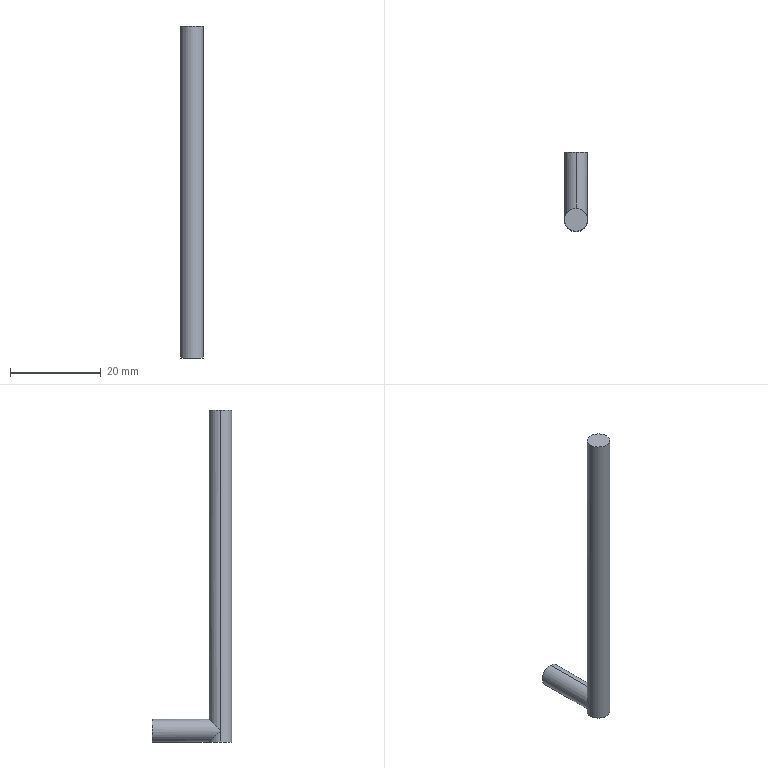Part | SolidWorks | features Extrusion 1, ICE 1 | 1 solid | 9 faces | box 5 x 17.5 x 73 mm | volume 1686 mm3 | cylinder 6 | plane 3 | commonest cylinder face diameters 5 x6
STEP:
#1=CARTESIAN_POINT('',(0.,15.,5.));
#2=VERTEX_POINT('',#1);
#3=CARTESIAN_POINT('',(0.,15.,0.));
#4=VERTEX_POINT('',#3);
#5=CARTESIAN_POINT('',(0.,15.,2.5));
#6=DIRECTION('',(0.,1.,0.));
#7=DIRECTION('',(0.,0.,1.));
#8=AXIS2_PLACEMENT_3D('',#5,#6,#7);
#9=CIRCLE('',#8,2.5);
#10=EDGE_CURVE('',#2,#4,#9,.T.);
#11=ORIENTED_EDGE('',*,*,#10,.F.);
#12=CARTESIAN_POINT('',(0.,2.5,5.));
#13=VERTEX_POINT('',#12);
#14=CARTESIAN_POINT('',(0.,15.,5.));
#15=DIRECTION('',(0.,-1.,0.));
#16=VECTOR('',#15,1000.);
#17=LINE('',#14,#16);
#18=EDGE_CURVE('',#2,#13,#17,.T.);
#19=ORIENTED_EDGE('',*,*,#18,.T.);
#20=CARTESIAN_POINT('',(2.5,0.,2.5));
#21=VERTEX_POINT('',#20);
#22=CARTESIAN_POINT('',(0.,2.5,5.));
#23=CARTESIAN_POINT('',(1.464,2.5,5.));
#24=CARTESIAN_POINT('',(2.5,1.464,3.964));
#25=CARTESIAN_POINT('',(2.5,0.,2.5));
#26=(BOUNDED_CURVE()B_SPLINE_CURVE(3,(#22,#23,#24,#25),.UNSPECIFIED.,.F.,.F.)B_SPLINE_CURVE_WITH_KNOTS((4,4),(3.142,4.712),.UNSPECIFIED.)CURVE()GEOMETRIC_REPRESENTATION_ITEM()RATIONAL_B_SPLINE_CURVE((1.,0.8047,0.8047,1.))REPRESENTATION_ITEM(''));
#27=EDGE_CURVE('',#13,#21,#26,.T.);
#28=ORIENTED_EDGE('',*,*,#27,.T.);
#29=CARTESIAN_POINT('',(0.,2.5,0.));
#30=VERTEX_POINT('',#29);
#31=CARTESIAN_POINT('',(2.5,0.,2.5));
#32=CARTESIAN_POINT('',(2.5,1.464,1.036));
#33=CARTESIAN_POINT('',(1.464,2.5,0.));
#34=CARTESIAN_POINT('',(0.,2.5,0.));
#35=(BOUNDED_CURVE()B_SPLINE_CURVE(3,(#31,#32,#33,#34),.UNSPECIFIED.,.F.,.T.)B_SPLINE_CURVE_WITH_KNOTS((4,4),(4.712,6.283),.UNSPECIFIED.)CURVE()GEOMETRIC_REPRESENTATION_ITEM()RATIONAL_B_SPLINE_CURVE((1.,0.8047,0.8047,1.))REPRESENTATION_ITEM(''));
#36=EDGE_CURVE('',#21,#30,#35,.T.);
#37=ORIENTED_EDGE('',*,*,#36,.T.);
#38=CARTESIAN_POINT('',(0.,15.,0.));
#39=DIRECTION('',(0.,-1.,0.));
#40=VECTOR('',#39,1000.);
#41=LINE('',#38,#40);
#42=EDGE_CURVE('',#4,#30,#41,.T.);
#43=ORIENTED_EDGE('',*,*,#42,.F.);
#44=EDGE_LOOP('',(#11,#19,#28,#37,#43));
#45=FACE_OUTER_BOUND('',#44,.T.);
#46=CARTESIAN_POINT('',(0.,15.,2.5));
#47=DIRECTION('',(0.,-1.,0.));
#48=DIRECTION('',(0.,0.,-1.));
#49=AXIS2_PLACEMENT_3D('',#46,#47,#48);
#50=CYLINDRICAL_SURFACE('',#49,2.5);
#51=ADVANCED_FACE('',(#45),#50,.T.);
#52=CARTESIAN_POINT('',(2.5,0.,73.));
#53=VERTEX_POINT('',#52);
#54=CARTESIAN_POINT('',(-2.5,0.,73.));
#55=VERTEX_POINT('',#54);
#56=CARTESIAN_POINT('',(0.,0.,73.));
#57=DIRECTION('',(0.,0.,1.));
#58=DIRECTION('',(1.,0.,0.));
#59=AXIS2_PLACEMENT_3D('',#56,#57,#58);
#60=CIRCLE('',#59,2.5);
#61=EDGE_CURVE('',#53,#55,#60,.T.);
#62=ORIENTED_EDGE('',*,*,#61,.F.);
#63=CARTESIAN_POINT('',(2.5,0.,73.));
#64=DIRECTION('',(0.,0.,-1.));
#65=VECTOR('',#64,1000.);
#66=LINE('',#63,#65);
#67=EDGE_CURVE('',#53,#21,#66,.T.);
#68=ORIENTED_EDGE('',*,*,#67,.T.);
#69=ORIENTED_EDGE('',*,*,#27,.F.);
#70=CARTESIAN_POINT('',(-2.5,0.,2.5));
#71=VERTEX_POINT('',#70);
#72=CARTESIAN_POINT('',(-2.5,0.,2.5));
#73=CARTESIAN_POINT('',(-2.5,1.464,3.964));
#74=CARTESIAN_POINT('',(-1.464,2.5,5.));
#75=CARTESIAN_POINT('',(0.,2.5,5.));
#76=(BOUNDED_CURVE()B_SPLINE_CURVE(3,(#72,#73,#74,#75),.UNSPECIFIED.,.F.,.F.)B_SPLINE_CURVE_WITH_KNOTS((4,4),(1.571,3.142),.UNSPECIFIED.)CURVE()GEOMETRIC_REPRESENTATION_ITEM()RATIONAL_B_SPLINE_CURVE((1.,0.8047,0.8047,1.))REPRESENTATION_ITEM(''));
#77=EDGE_CURVE('',#71,#13,#76,.T.);
#78=ORIENTED_EDGE('',*,*,#77,.F.);
#79=CARTESIAN_POINT('',(-2.5,0.,73.));
#80=DIRECTION('',(0.,0.,-1.));
#81=VECTOR('',#80,1000.);
#82=LINE('',#79,#81);
#83=EDGE_CURVE('',#55,#71,#82,.T.);
#84=ORIENTED_EDGE('',*,*,#83,.F.);
#85=EDGE_LOOP('',(#62,#68,#69,#78,#84));
#86=FACE_OUTER_BOUND('',#85,.T.);
#87=CARTESIAN_POINT('',(0.,0.,73.));
#88=DIRECTION('',(0.,0.,-1.));
#89=DIRECTION('',(-1.,0.,0.));
#90=AXIS2_PLACEMENT_3D('',#87,#88,#89);
#91=CYLINDRICAL_SURFACE('',#90,2.5);
#92=ADVANCED_FACE('',(#86),#91,.T.);
#93=ORIENTED_EDGE('',*,*,#36,.F.);
#94=CARTESIAN_POINT('',(2.5,0.,0.));
#95=VERTEX_POINT('',#94);
#96=CARTESIAN_POINT('',(2.5,0.,73.));
#97=DIRECTION('',(0.,0.,-1.));
#98=VECTOR('',#97,1000.);
#99=LINE('',#96,#98);
#100=EDGE_CURVE('',#21,#95,#99,.T.);
#101=ORIENTED_EDGE('',*,*,#100,.T.);
#102=CARTESIAN_POINT('',(0.,0.,0.));
#103=DIRECTION('',(0.,0.,1.));
#104=DIRECTION('',(1.,0.,0.));
#105=AXIS2_PLACEMENT_3D('',#102,#103,#104);
#106=CIRCLE('',#105,2.5);
#107=EDGE_CURVE('',#95,#30,#106,.T.);
#108=ORIENTED_EDGE('',*,*,#107,.T.);
#109=EDGE_LOOP('',(#93,#101,#108));
#110=FACE_OUTER_BOUND('',#109,.T.);
#111=CARTESIAN_POINT('',(0.,0.,73.));
#112=DIRECTION('',(0.,0.,-1.));
#113=DIRECTION('',(-1.,0.,0.));
#114=AXIS2_PLACEMENT_3D('',#111,#112,#113);
#115=CYLINDRICAL_SURFACE('',#114,2.5);
#116=ADVANCED_FACE('',(#110),#115,.T.);
#117=ORIENTED_EDGE('',*,*,#67,.F.);
#118=CARTESIAN_POINT('',(0.,0.,73.));
#119=DIRECTION('',(0.,0.,1.));
#120=DIRECTION('',(1.,0.,0.));
#121=AXIS2_PLACEMENT_3D('',#118,#119,#120);
#122=CIRCLE('',#121,2.5);
#123=EDGE_CURVE('',#55,#53,#122,.T.);
#124=ORIENTED_EDGE('',*,*,#123,.F.);
#125=ORIENTED_EDGE('',*,*,#83,.T.);
#126=CARTESIAN_POINT('',(-2.5,0.,0.));
#127=VERTEX_POINT('',#126);
#128=CARTESIAN_POINT('',(-2.5,0.,73.));
#129=DIRECTION('',(0.,0.,-1.));
#130=VECTOR('',#129,1000.);
#131=LINE('',#128,#130);
#132=EDGE_CURVE('',#71,#127,#131,.T.);
#133=ORIENTED_EDGE('',*,*,#132,.T.);
#134=CARTESIAN_POINT('',(0.,0.,0.));
#135=DIRECTION('',(0.,0.,1.));
#136=DIRECTION('',(1.,0.,0.));
#137=AXIS2_PLACEMENT_3D('',#134,#135,#136);
#138=CIRCLE('',#137,2.5);
#139=EDGE_CURVE('',#127,#95,#138,.T.);
#140=ORIENTED_EDGE('',*,*,#139,.T.);
#141=ORIENTED_EDGE('',*,*,#100,.F.);
#142=EDGE_LOOP('',(#117,#124,#125,#133,#140,#141));
#143=FACE_OUTER_BOUND('',#142,.T.);
#144=CARTESIAN_POINT('',(0.,0.,73.));
#145=DIRECTION('',(0.,0.,-1.));
#146=DIRECTION('',(-1.,0.,0.));
#147=AXIS2_PLACEMENT_3D('',#144,#145,#146);
#148=CYLINDRICAL_SURFACE('',#147,2.5);
#149=ADVANCED_FACE('',(#143),#148,.T.);
#150=ORIENTED_EDGE('',*,*,#132,.F.);
#151=CARTESIAN_POINT('',(0.,2.5,0.));
#152=CARTESIAN_POINT('',(-1.464,2.5,0.));
#153=CARTESIAN_POINT('',(-2.5,1.464,1.036));
#154=CARTESIAN_POINT('',(-2.5,0.,2.5));
#155=(BOUNDED_CURVE()B_SPLINE_CURVE(3,(#151,#152,#153,#154),.UNSPECIFIED.,.F.,.F.)B_SPLINE_CURVE_WITH_KNOTS((4,4),(0.,1.571),.UNSPECIFIED.)CURVE()GEOMETRIC_REPRESENTATION_ITEM()RATIONAL_B_SPLINE_CURVE((1.,0.8047,0.8047,1.))REPRESENTATION_ITEM(''));
#156=EDGE_CURVE('',#30,#71,#155,.T.);
#157=ORIENTED_EDGE('',*,*,#156,.F.);
#158=CARTESIAN_POINT('',(0.,0.,0.));
#159=DIRECTION('',(0.,0.,1.));
#160=DIRECTION('',(1.,0.,0.));
#161=AXIS2_PLACEMENT_3D('',#158,#159,#160);
#162=CIRCLE('',#161,2.5);
#163=EDGE_CURVE('',#30,#127,#162,.T.);
#164=ORIENTED_EDGE('',*,*,#163,.T.);
#165=EDGE_LOOP('',(#150,#157,#164));
#166=FACE_OUTER_BOUND('',#165,.T.);
#167=CARTESIAN_POINT('',(0.,0.,73.));
#168=DIRECTION('',(0.,0.,-1.));
#169=DIRECTION('',(-1.,0.,0.));
#170=AXIS2_PLACEMENT_3D('',#167,#168,#169);
#171=CYLINDRICAL_SURFACE('',#170,2.5);
#172=ADVANCED_FACE('',(#166),#171,.T.);
#173=ORIENTED_EDGE('',*,*,#123,.T.);
#174=ORIENTED_EDGE('',*,*,#61,.T.);
#175=EDGE_LOOP('',(#173,#174));
#176=FACE_OUTER_BOUND('',#175,.T.);
#177=CARTESIAN_POINT('',(0.,0.,73.));
#178=DIRECTION('',(0.,0.,1.));
#179=DIRECTION('',(1.,0.,0.));
#180=AXIS2_PLACEMENT_3D('',#177,#178,#179);
#181=PLANE('',#180);
#182=ADVANCED_FACE('',(#176),#181,.T.);
#183=ORIENTED_EDGE('',*,*,#163,.F.);
#184=ORIENTED_EDGE('',*,*,#107,.F.);
#185=ORIENTED_EDGE('',*,*,#139,.F.);
#186=EDGE_LOOP('',(#183,#184,#185));
#187=FACE_OUTER_BOUND('',#186,.T.);
#188=CARTESIAN_POINT('',(0.,0.,0.));
#189=DIRECTION('',(0.,0.,1.));
#190=DIRECTION('',(1.,0.,0.));
#191=AXIS2_PLACEMENT_3D('',#188,#189,#190);
#192=PLANE('',#191);
#193=ADVANCED_FACE('',(#187),#192,.F.);
#194=ORIENTED_EDGE('',*,*,#18,.F.);
#195=CARTESIAN_POINT('',(0.,15.,2.5));
#196=DIRECTION('',(0.,1.,0.));
#197=DIRECTION('',(0.,0.,1.));
#198=AXIS2_PLACEMENT_3D('',#195,#196,#197);
#199=CIRCLE('',#198,2.5);
#200=EDGE_CURVE('',#4,#2,#199,.T.);
#201=ORIENTED_EDGE('',*,*,#200,.F.);
#202=ORIENTED_EDGE('',*,*,#42,.T.);
#203=ORIENTED_EDGE('',*,*,#156,.T.);
#204=ORIENTED_EDGE('',*,*,#77,.T.);
#205=EDGE_LOOP('',(#194,#201,#202,#203,#204));
#206=FACE_OUTER_BOUND('',#205,.T.);
#207=CARTESIAN_POINT('',(0.,15.,2.5));
#208=DIRECTION('',(0.,-1.,0.));
#209=DIRECTION('',(0.,0.,-1.));
#210=AXIS2_PLACEMENT_3D('',#207,#208,#209);
#211=CYLINDRICAL_SURFACE('',#210,2.5);
#212=ADVANCED_FACE('',(#206),#211,.T.);
#213=ORIENTED_EDGE('',*,*,#200,.T.);
#214=ORIENTED_EDGE('',*,*,#10,.T.);
#215=EDGE_LOOP('',(#213,#214));
#216=FACE_OUTER_BOUND('',#215,.T.);
#217=CARTESIAN_POINT('',(0.,15.,2.5));
#218=DIRECTION('',(0.,1.,0.));
#219=DIRECTION('',(0.,0.,1.));
#220=AXIS2_PLACEMENT_3D('',#217,#218,#219);
#221=PLANE('',#220);
#222=ADVANCED_FACE('',(#216),#221,.T.);
#223=CLOSED_SHELL('',(#51,#92,#116,#149,#172,#182,#193,#212,#222));
#224=MANIFOLD_SOLID_BREP('',#223);
#225=CARTESIAN_POINT('',(0.,0.,0.));
#226=DIRECTION('',(0.,0.,1.));
#227=DIRECTION('',(1.,0.,0.));
#228=AXIS2_PLACEMENT_3D('',#225,#226,#227);
#229=(LENGTH_UNIT()NAMED_UNIT(*)SI_UNIT(.MILLI.,.METRE.));
#230=UNCERTAINTY_MEASURE_WITH_UNIT(LENGTH_MEASURE(0.00001),#229,'','');
#231=(NAMED_UNIT(*)PLANE_ANGLE_UNIT()SI_UNIT($,.RADIAN.));
#232=(NAMED_UNIT(*)SI_UNIT($,.STERADIAN.)SOLID_ANGLE_UNIT());
#233=(GEOMETRIC_REPRESENTATION_CONTEXT(3)GLOBAL_UNCERTAINTY_ASSIGNED_CONTEXT((#230))GLOBAL_UNIT_ASSIGNED_CONTEXT((#229,#231,#232))REPRESENTATION_CONTEXT('',''));
#234=ADVANCED_BREP_SHAPE_REPRESENTATION('',(#224,#228),#233);